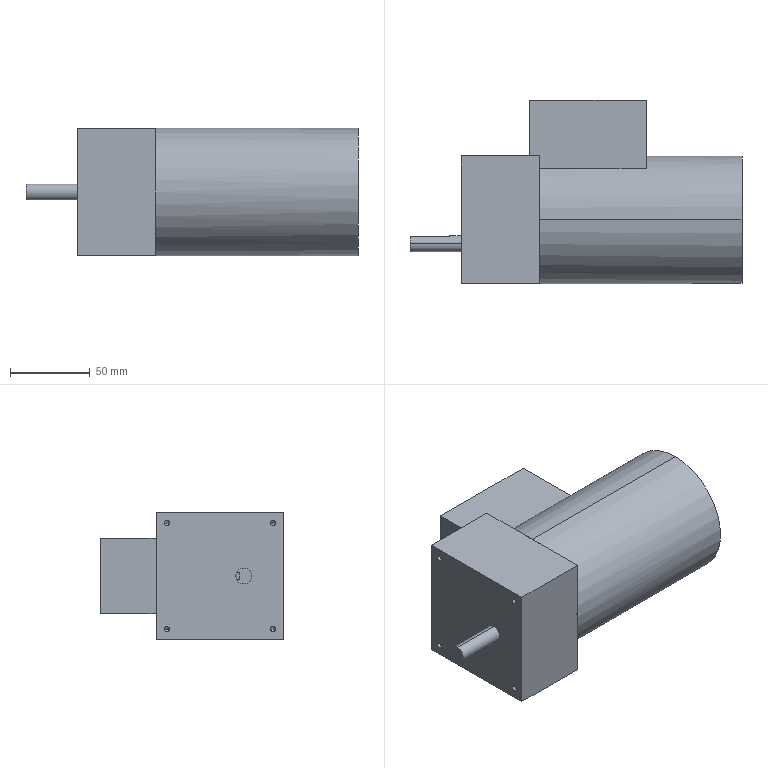Part | STEP file | Motor JSCC 25W | 1 solid | 40 faces | box 208 x 115 x 80 mm | volume 1081551 mm3 | plane 20 | cylinder 12 | cone 8 | commonest cylinder face diameters 3.3 x8 10 x2 80 x2